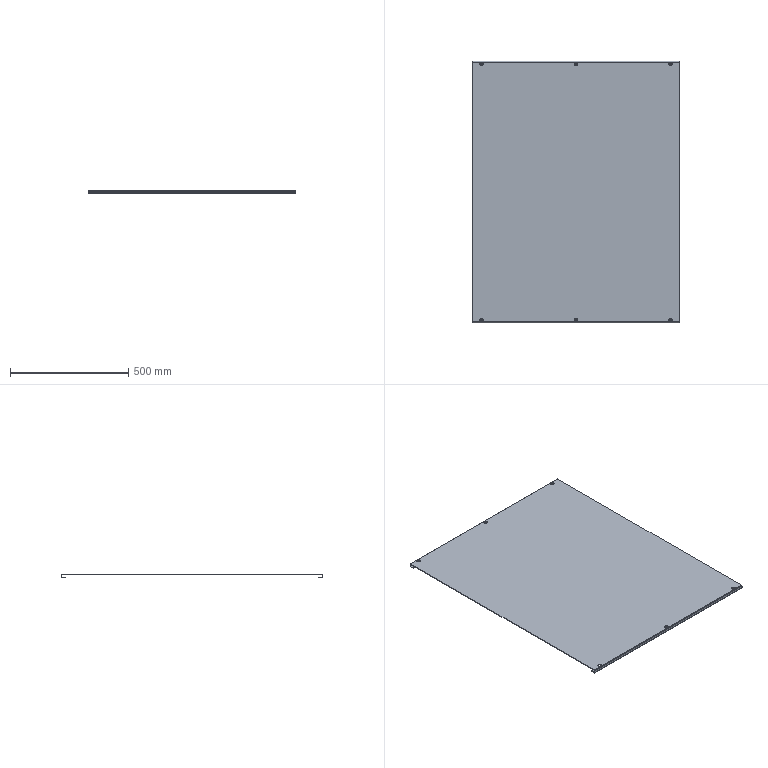Part | STEP file | Support steel plate | 1 solid | 62 faces | box 880 x 1107 x 15.737 mm | volume 3066275 mm3 | cylinder 32 | plane 30 | commonest cylinder face diameters 9 x12 15 x12 1.473 x4 7.473 x4